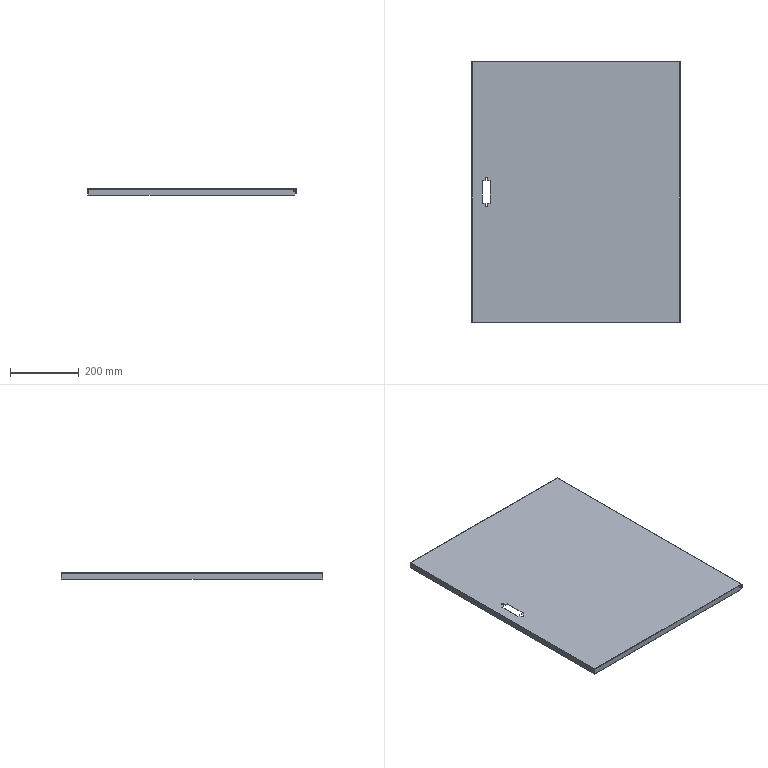Part | SolidWorks | features ICE 4, CornerFeat 1, EdgeFlange 1, FlatPattern 1, SMBaseFlange 1, SheetMetal 1 | 1 solid | 56 faces | box 605 x 758 x 18 mm | volume 498938 mm3 | plane 38 | cylinder 14 | spline 4 | commonest cylinder face diameters 0.4 x4 2.4 x4 4.5 x2 6 x2 7 x2